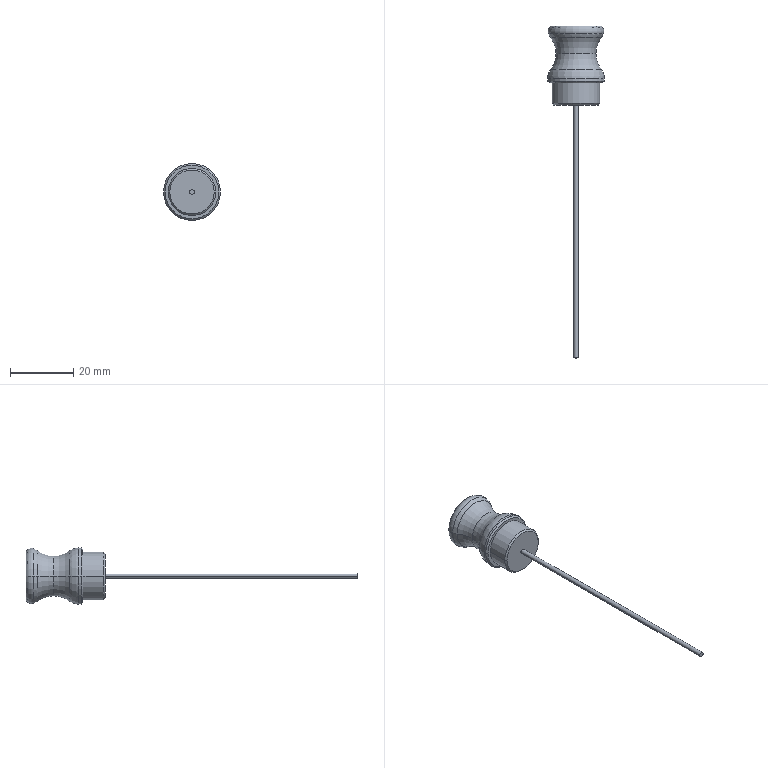Part | SolidWorks | features Chamfer 2, Fillet 1, Revolution 1 | 1 solid | 26 faces | box 18 x 105 x 18 mm | volume 4726 mm3 | torus 10 | cone 6 | cylinder 6 | plane 4 | commonest cylinder face diameters 1.5 x2 15 x2 18 x2
STEP:
#1=CARTESIAN_POINT('',(7.995,11.261,0.));
#2=VERTEX_POINT('',#1);
#3=CARTESIAN_POINT('',(6.308,16.305,0.));
#4=VERTEX_POINT('',#3);
#5=CARTESIAN_POINT('',(14.695,16.305,0.));
#6=DIRECTION('',(0.,0.,-1.));
#7=DIRECTION('',(-1.,0.,0.));
#8=AXIS2_PLACEMENT_3D('',#5,#6,#7);
#9=CIRCLE('',#8,8.387);
#10=EDGE_CURVE('',#2,#4,#9,.T.);
#11=ORIENTED_EDGE('',*,*,#10,.T.);
#12=CARTESIAN_POINT('',(-6.308,16.305,0.));
#13=VERTEX_POINT('',#12);
#14=CARTESIAN_POINT('',(0.,16.305,0.));
#15=DIRECTION('',(0.,-1.,0.));
#16=DIRECTION('',(1.,0.,0.));
#17=AXIS2_PLACEMENT_3D('',#14,#15,#16);
#18=CIRCLE('',#17,6.308);
#19=EDGE_CURVE('',#4,#13,#18,.T.);
#20=ORIENTED_EDGE('',*,*,#19,.T.);
#21=CARTESIAN_POINT('',(-7.995,11.261,0.));
#22=VERTEX_POINT('',#21);
#23=CARTESIAN_POINT('',(-14.695,16.305,0.));
#24=DIRECTION('',(0.,0.,1.));
#25=DIRECTION('',(1.,0.,0.));
#26=AXIS2_PLACEMENT_3D('',#23,#24,#25);
#27=CIRCLE('',#26,8.387);
#28=EDGE_CURVE('',#22,#13,#27,.T.);
#29=ORIENTED_EDGE('',*,*,#28,.F.);
#30=CARTESIAN_POINT('',(0.,11.261,0.));
#31=DIRECTION('',(0.,-1.,0.));
#32=DIRECTION('',(1.,0.,0.));
#33=AXIS2_PLACEMENT_3D('',#30,#31,#32);
#34=CIRCLE('',#33,7.995);
#35=EDGE_CURVE('',#2,#22,#34,.T.);
#36=ORIENTED_EDGE('',*,*,#35,.F.);
#37=EDGE_LOOP('',(#11,#20,#29,#36));
#38=FACE_OUTER_BOUND('',#37,.T.);
#39=CARTESIAN_POINT('',(0.,16.305,0.));
#40=DIRECTION('',(0.,-1.,0.));
#41=DIRECTION('',(1.,0.,0.));
#42=AXIS2_PLACEMENT_3D('',#39,#40,#41);
#43=TOROIDAL_SURFACE('',#42,14.695,8.387);
#44=ADVANCED_FACE('',(#38),#43,.F.);
#45=ORIENTED_EDGE('',*,*,#28,.T.);
#46=CARTESIAN_POINT('',(0.,16.305,0.));
#47=DIRECTION('',(0.,-1.,0.));
#48=DIRECTION('',(1.,0.,0.));
#49=AXIS2_PLACEMENT_3D('',#46,#47,#48);
#50=CIRCLE('',#49,6.308);
#51=EDGE_CURVE('',#13,#4,#50,.T.);
#52=ORIENTED_EDGE('',*,*,#51,.T.);
#53=ORIENTED_EDGE('',*,*,#10,.F.);
#54=CARTESIAN_POINT('',(0.,11.261,0.));
#55=DIRECTION('',(0.,-1.,0.));
#56=DIRECTION('',(1.,0.,0.));
#57=AXIS2_PLACEMENT_3D('',#54,#55,#56);
#58=CIRCLE('',#57,7.995);
#59=EDGE_CURVE('',#22,#2,#58,.T.);
#60=ORIENTED_EDGE('',*,*,#59,.F.);
#61=EDGE_LOOP('',(#45,#52,#53,#60));
#62=FACE_OUTER_BOUND('',#61,.T.);
#63=CARTESIAN_POINT('',(0.,16.305,0.));
#64=DIRECTION('',(0.,-1.,0.));
#65=DIRECTION('',(1.,0.,0.));
#66=AXIS2_PLACEMENT_3D('',#63,#64,#65);
#67=TOROIDAL_SURFACE('',#66,14.695,8.387);
#68=ADVANCED_FACE('',(#62),#67,.F.);
#69=CARTESIAN_POINT('',(8.69,22.623,0.));
#70=VERTEX_POINT('',#69);
#71=CARTESIAN_POINT('',(-8.69,22.623,0.));
#72=VERTEX_POINT('',#71);
#73=CARTESIAN_POINT('',(0.,22.623,0.));
#74=DIRECTION('',(0.,-1.,0.));
#75=DIRECTION('',(-1.,0.,0.));
#76=AXIS2_PLACEMENT_3D('',#73,#74,#75);
#77=CIRCLE('',#76,8.69);
#78=EDGE_CURVE('',#70,#72,#77,.T.);
#79=ORIENTED_EDGE('',*,*,#78,.F.);
#80=CARTESIAN_POINT('',(8.29,24.666,0.));
#81=VERTEX_POINT('',#80);
#82=CARTESIAN_POINT('',(6.814,23.316,0.));
#83=DIRECTION('',(0.,0.,1.));
#84=DIRECTION('',(1.,0.,0.));
#85=AXIS2_PLACEMENT_3D('',#82,#83,#84);
#86=CIRCLE('',#85,2.);
#87=EDGE_CURVE('',#70,#81,#86,.T.);
#88=ORIENTED_EDGE('',*,*,#87,.T.);
#89=CARTESIAN_POINT('',(-8.29,24.666,0.));
#90=VERTEX_POINT('',#89);
#91=CARTESIAN_POINT('',(0.,24.666,0.));
#92=DIRECTION('',(0.,1.,0.));
#93=DIRECTION('',(-1.,0.,0.));
#94=AXIS2_PLACEMENT_3D('',#91,#92,#93);
#95=CIRCLE('',#94,8.29);
#96=EDGE_CURVE('',#90,#81,#95,.T.);
#97=ORIENTED_EDGE('',*,*,#96,.F.);
#98=CARTESIAN_POINT('',(-6.814,23.316,0.));
#99=DIRECTION('',(0.,0.,-1.));
#100=DIRECTION('',(-1.,0.,0.));
#101=AXIS2_PLACEMENT_3D('',#98,#99,#100);
#102=CIRCLE('',#101,2.);
#103=EDGE_CURVE('',#72,#90,#102,.T.);
#104=ORIENTED_EDGE('',*,*,#103,.F.);
#105=EDGE_LOOP('',(#79,#88,#97,#104));
#106=FACE_OUTER_BOUND('',#105,.T.);
#107=CARTESIAN_POINT('',(0.,23.316,0.));
#108=DIRECTION('',(0.,1.,0.));
#109=DIRECTION('',(-1.,0.,0.));
#110=AXIS2_PLACEMENT_3D('',#107,#108,#109);
#111=TOROIDAL_SURFACE('',#110,6.814,2.);
#112=ADVANCED_FACE('',(#106),#111,.T.);
#113=CARTESIAN_POINT('',(7.,0.,0.));
#114=VERTEX_POINT('',#113);
#115=CARTESIAN_POINT('',(-7.,0.,0.));
#116=VERTEX_POINT('',#115);
#117=CARTESIAN_POINT('',(0.,0.,0.));
#118=DIRECTION('',(0.,-1.,0.));
#119=DIRECTION('',(1.,0.,0.));
#120=AXIS2_PLACEMENT_3D('',#117,#118,#119);
#121=CIRCLE('',#120,7.);
#122=EDGE_CURVE('',#114,#116,#121,.T.);
#123=ORIENTED_EDGE('',*,*,#122,.F.);
#124=CARTESIAN_POINT('',(7.5,0.5,0.));
#125=VERTEX_POINT('',#124);
#126=CARTESIAN_POINT('',(7.,0.,0.));
#127=DIRECTION('',(0.7071,0.7071,0.));
#128=VECTOR('',#127,1000.);
#129=LINE('',#126,#128);
#130=EDGE_CURVE('',#114,#125,#129,.T.);
#131=ORIENTED_EDGE('',*,*,#130,.T.);
#132=CARTESIAN_POINT('',(-7.5,0.5,0.));
#133=VERTEX_POINT('',#132);
#134=CARTESIAN_POINT('',(0.,0.5,0.));
#135=DIRECTION('',(0.,1.,0.));
#136=DIRECTION('',(1.,0.,0.));
#137=AXIS2_PLACEMENT_3D('',#134,#135,#136);
#138=CIRCLE('',#137,7.5);
#139=EDGE_CURVE('',#133,#125,#138,.T.);
#140=ORIENTED_EDGE('',*,*,#139,.F.);
#141=CARTESIAN_POINT('',(-7.,0.,0.));
#142=DIRECTION('',(-0.7071,0.7071,0.));
#143=VECTOR('',#142,1000.);
#144=LINE('',#141,#143);
#145=EDGE_CURVE('',#116,#133,#144,.T.);
#146=ORIENTED_EDGE('',*,*,#145,.F.);
#147=EDGE_LOOP('',(#123,#131,#140,#146));
#148=FACE_OUTER_BOUND('',#147,.T.);
#149=CARTESIAN_POINT('',(0.,0.,0.));
#150=DIRECTION('',(0.,1.,0.));
#151=DIRECTION('',(-1.,0.,0.));
#152=AXIS2_PLACEMENT_3D('',#149,#150,#151);
#153=CONICAL_SURFACE('',#152,7.,0.7854);
#154=ADVANCED_FACE('',(#148),#153,.T.);
#155=CARTESIAN_POINT('',(8.5,7.,0.));
#156=VERTEX_POINT('',#155);
#157=CARTESIAN_POINT('',(-8.5,7.,0.));
#158=VERTEX_POINT('',#157);
#159=CARTESIAN_POINT('',(0.,7.,0.));
#160=DIRECTION('',(0.,-1.,0.));
#161=DIRECTION('',(1.,0.,0.));
#162=AXIS2_PLACEMENT_3D('',#159,#160,#161);
#163=CIRCLE('',#162,8.5);
#164=EDGE_CURVE('',#156,#158,#163,.T.);
#165=ORIENTED_EDGE('',*,*,#164,.F.);
#166=CARTESIAN_POINT('',(9.,7.5,0.));
#167=VERTEX_POINT('',#166);
#168=CARTESIAN_POINT('',(8.5,7.,0.));
#169=DIRECTION('',(0.7071,0.7071,0.));
#170=VECTOR('',#169,1000.);
#171=LINE('',#168,#170);
#172=EDGE_CURVE('',#156,#167,#171,.T.);
#173=ORIENTED_EDGE('',*,*,#172,.T.);
#174=CARTESIAN_POINT('',(-9.,7.5,0.));
#175=VERTEX_POINT('',#174);
#176=CARTESIAN_POINT('',(0.,7.5,0.));
#177=DIRECTION('',(0.,1.,0.));
#178=DIRECTION('',(1.,0.,0.));
#179=AXIS2_PLACEMENT_3D('',#176,#177,#178);
#180=CIRCLE('',#179,9.);
#181=EDGE_CURVE('',#175,#167,#180,.T.);
#182=ORIENTED_EDGE('',*,*,#181,.F.);
#183=CARTESIAN_POINT('',(-8.5,7.,0.));
#184=DIRECTION('',(-0.7071,0.7071,0.));
#185=VECTOR('',#184,1000.);
#186=LINE('',#183,#185);
#187=EDGE_CURVE('',#158,#175,#186,.T.);
#188=ORIENTED_EDGE('',*,*,#187,.F.);
#189=EDGE_LOOP('',(#165,#173,#182,#188));
#190=FACE_OUTER_BOUND('',#189,.T.);
#191=CARTESIAN_POINT('',(0.,7.,0.));
#192=DIRECTION('',(0.,1.,0.));
#193=DIRECTION('',(-1.,0.,0.));
#194=AXIS2_PLACEMENT_3D('',#191,#192,#193);
#195=CONICAL_SURFACE('',#194,8.5,0.7854);
#196=ADVANCED_FACE('',(#190),#195,.T.);
#197=CARTESIAN_POINT('',(-7.984,25.,0.));
#198=VERTEX_POINT('',#197);
#199=CARTESIAN_POINT('',(7.984,25.,0.));
#200=VERTEX_POINT('',#199);
#201=CARTESIAN_POINT('',(0.,25.,0.));
#202=DIRECTION('',(0.,1.,0.));
#203=DIRECTION('',(-1.,0.,0.));
#204=AXIS2_PLACEMENT_3D('',#201,#202,#203);
#205=CIRCLE('',#204,7.984);
#206=EDGE_CURVE('',#198,#200,#205,.T.);
#207=ORIENTED_EDGE('',*,*,#206,.F.);
#208=CARTESIAN_POINT('',(-8.98,23.911,0.));
#209=DIRECTION('',(-0.675,-0.7379,0.));
#210=VECTOR('',#209,1000.);
#211=LINE('',#208,#210);
#212=EDGE_CURVE('',#198,#90,#211,.T.);
#213=ORIENTED_EDGE('',*,*,#212,.T.);
#214=ORIENTED_EDGE('',*,*,#96,.T.);
#215=CARTESIAN_POINT('',(8.98,23.911,0.));
#216=DIRECTION('',(0.675,-0.7379,0.));
#217=VECTOR('',#216,1000.);
#218=LINE('',#215,#217);
#219=EDGE_CURVE('',#200,#81,#218,.T.);
#220=ORIENTED_EDGE('',*,*,#219,.F.);
#221=EDGE_LOOP('',(#207,#213,#214,#220));
#222=FACE_OUTER_BOUND('',#221,.T.);
#223=CARTESIAN_POINT('',(0.,23.911,0.));
#224=DIRECTION('',(0.,-1.,0.));
#225=DIRECTION('',(1.,0.,0.));
#226=AXIS2_PLACEMENT_3D('',#223,#224,#225);
#227=CONICAL_SURFACE('',#226,8.98,0.7409);
#228=ADVANCED_FACE('',(#222),#227,.T.);
#229=CARTESIAN_POINT('',(0.75,0.,0.));
#230=VERTEX_POINT('',#229);
#231=CARTESIAN_POINT('',(-0.75,0.,0.));
#232=VERTEX_POINT('',#231);
#233=CARTESIAN_POINT('',(0.,0.,0.));
#234=DIRECTION('',(0.,-1.,0.));
#235=DIRECTION('',(1.,0.,0.));
#236=AXIS2_PLACEMENT_3D('',#233,#234,#235);
#237=CIRCLE('',#236,0.75);
#238=EDGE_CURVE('',#230,#232,#237,.T.);
#239=ORIENTED_EDGE('',*,*,#238,.T.);
#240=CARTESIAN_POINT('',(-0.75,-80.,0.));
#241=VERTEX_POINT('',#240);
#242=CARTESIAN_POINT('',(-0.75,-80.,0.));
#243=DIRECTION('',(0.,-1.,0.));
#244=VECTOR('',#243,1000.);
#245=LINE('',#242,#244);
#246=EDGE_CURVE('',#232,#241,#245,.T.);
#247=ORIENTED_EDGE('',*,*,#246,.T.);
#248=CARTESIAN_POINT('',(0.75,-80.,0.));
#249=VERTEX_POINT('',#248);
#250=CARTESIAN_POINT('',(0.,-80.,0.));
#251=DIRECTION('',(0.,-1.,0.));
#252=DIRECTION('',(1.,0.,0.));
#253=AXIS2_PLACEMENT_3D('',#250,#251,#252);
#254=CIRCLE('',#253,0.75);
#255=EDGE_CURVE('',#249,#241,#254,.T.);
#256=ORIENTED_EDGE('',*,*,#255,.F.);
#257=CARTESIAN_POINT('',(0.75,-80.,0.));
#258=DIRECTION('',(0.,-1.,0.));
#259=VECTOR('',#258,1000.);
#260=LINE('',#257,#259);
#261=EDGE_CURVE('',#230,#249,#260,.T.);
#262=ORIENTED_EDGE('',*,*,#261,.F.);
#263=EDGE_LOOP('',(#239,#247,#256,#262));
#264=FACE_OUTER_BOUND('',#263,.T.);
#265=CARTESIAN_POINT('',(0.,-80.,0.));
#266=DIRECTION('',(0.,-1.,0.));
#267=DIRECTION('',(1.,0.,0.));
#268=AXIS2_PLACEMENT_3D('',#265,#266,#267);
#269=CYLINDRICAL_SURFACE('',#268,0.75);
#270=ADVANCED_FACE('',(#264),#269,.T.);
#271=ORIENTED_EDGE('',*,*,#78,.T.);
#272=CARTESIAN_POINT('',(-7.995,21.348,0.));
#273=VERTEX_POINT('',#272);
#274=CARTESIAN_POINT('',(-4.,24.355,0.));
#275=DIRECTION('',(0.,0.,1.));
#276=DIRECTION('',(1.,0.,0.));
#277=AXIS2_PLACEMENT_3D('',#274,#275,#276);
#278=CIRCLE('',#277,5.);
#279=EDGE_CURVE('',#72,#273,#278,.T.);
#280=ORIENTED_EDGE('',*,*,#279,.T.);
#281=CARTESIAN_POINT('',(7.995,21.348,0.));
#282=VERTEX_POINT('',#281);
#283=CARTESIAN_POINT('',(0.,21.348,0.));
#284=DIRECTION('',(0.,-1.,0.));
#285=DIRECTION('',(1.,0.,0.));
#286=AXIS2_PLACEMENT_3D('',#283,#284,#285);
#287=CIRCLE('',#286,7.995);
#288=EDGE_CURVE('',#282,#273,#287,.T.);
#289=ORIENTED_EDGE('',*,*,#288,.F.);
#290=CARTESIAN_POINT('',(4.,24.355,0.));
#291=DIRECTION('',(0.,0.,-1.));
#292=DIRECTION('',(-1.,0.,0.));
#293=AXIS2_PLACEMENT_3D('',#290,#291,#292);
#294=CIRCLE('',#293,5.);
#295=EDGE_CURVE('',#70,#282,#294,.T.);
#296=ORIENTED_EDGE('',*,*,#295,.F.);
#297=EDGE_LOOP('',(#271,#280,#289,#296));
#298=FACE_OUTER_BOUND('',#297,.T.);
#299=CARTESIAN_POINT('',(0.,24.355,0.));
#300=DIRECTION('',(0.,-1.,0.));
#301=DIRECTION('',(1.,0.,0.));
#302=AXIS2_PLACEMENT_3D('',#299,#300,#301);
#303=TOROIDAL_SURFACE('',#302,4.,5.);
#304=ADVANCED_FACE('',(#298),#303,.T.);
#305=ORIENTED_EDGE('',*,*,#51,.F.);
#306=CARTESIAN_POINT('',(-14.695,16.305,0.));
#307=DIRECTION('',(0.,0.,1.));
#308=DIRECTION('',(1.,0.,0.));
#309=AXIS2_PLACEMENT_3D('',#306,#307,#308);
#310=CIRCLE('',#309,8.387);
#311=EDGE_CURVE('',#13,#273,#310,.T.);
#312=ORIENTED_EDGE('',*,*,#311,.T.);
#313=CARTESIAN_POINT('',(0.,21.348,0.));
#314=DIRECTION('',(0.,-1.,0.));
#315=DIRECTION('',(1.,0.,0.));
#316=AXIS2_PLACEMENT_3D('',#313,#314,#315);
#317=CIRCLE('',#316,7.995);
#318=EDGE_CURVE('',#273,#282,#317,.T.);
#319=ORIENTED_EDGE('',*,*,#318,.T.);
#320=CARTESIAN_POINT('',(14.695,16.305,0.));
#321=DIRECTION('',(0.,0.,-1.));
#322=DIRECTION('',(-1.,0.,0.));
#323=AXIS2_PLACEMENT_3D('',#320,#321,#322);
#324=CIRCLE('',#323,8.387);
#325=EDGE_CURVE('',#4,#282,#324,.T.);
#326=ORIENTED_EDGE('',*,*,#325,.F.);
#327=EDGE_LOOP('',(#305,#312,#319,#326));
#328=FACE_OUTER_BOUND('',#327,.T.);
#329=CARTESIAN_POINT('',(0.,16.305,0.));
#330=DIRECTION('',(0.,-1.,0.));
#331=DIRECTION('',(1.,0.,0.));
#332=AXIS2_PLACEMENT_3D('',#329,#330,#331);
#333=TOROIDAL_SURFACE('',#332,14.695,8.387);
#334=ADVANCED_FACE('',(#328),#333,.F.);
#335=ORIENTED_EDGE('',*,*,#35,.T.);
#336=CARTESIAN_POINT('',(-9.,8.254,0.));
#337=VERTEX_POINT('',#336);
#338=CARTESIAN_POINT('',(-4.,8.254,0.));
#339=DIRECTION('',(0.,0.,1.));
#340=DIRECTION('',(1.,0.,0.));
#341=AXIS2_PLACEMENT_3D('',#338,#339,#340);
#342=CIRCLE('',#341,5.);
#343=EDGE_CURVE('',#22,#337,#342,.T.);
#344=ORIENTED_EDGE('',*,*,#343,.T.);
#345=CARTESIAN_POINT('',(9.,8.254,0.));
#346=VERTEX_POINT('',#345);
#347=CARTESIAN_POINT('',(0.,8.254,0.));
#348=DIRECTION('',(0.,-1.,0.));
#349=DIRECTION('',(1.,0.,0.));
#350=AXIS2_PLACEMENT_3D('',#347,#348,#349);
#351=CIRCLE('',#350,9.);
#352=EDGE_CURVE('',#346,#337,#351,.T.);
#353=ORIENTED_EDGE('',*,*,#352,.F.);
#354=CARTESIAN_POINT('',(4.,8.254,0.));
#355=DIRECTION('',(0.,0.,-1.));
#356=DIRECTION('',(-1.,0.,0.));
#357=AXIS2_PLACEMENT_3D('',#354,#355,#356);
#358=CIRCLE('',#357,5.);
#359=EDGE_CURVE('',#2,#346,#358,.T.);
#360=ORIENTED_EDGE('',*,*,#359,.F.);
#361=EDGE_LOOP('',(#335,#344,#353,#360));
#362=FACE_OUTER_BOUND('',#361,.T.);
#363=CARTESIAN_POINT('',(0.,8.254,0.));
#364=DIRECTION('',(0.,-1.,0.));
#365=DIRECTION('',(1.,0.,0.));
#366=AXIS2_PLACEMENT_3D('',#363,#364,#365);
#367=TOROIDAL_SURFACE('',#366,4.,5.);
#368=ADVANCED_FACE('',(#362),#367,.T.);
#369=ORIENTED_EDGE('',*,*,#352,.T.);
#370=CARTESIAN_POINT('',(-9.,-80.,0.));
#371=DIRECTION('',(0.,-1.,0.));
#372=VECTOR('',#371,1000.);
#373=LINE('',#370,#372);
#374=EDGE_CURVE('',#337,#175,#373,.T.);
#375=ORIENTED_EDGE('',*,*,#374,.T.);
#376=ORIENTED_EDGE('',*,*,#181,.T.);
#377=CARTESIAN_POINT('',(9.,-80.,0.));
#378=DIRECTION('',(0.,-1.,0.));
#379=VECTOR('',#378,1000.);
#380=LINE('',#377,#379);
#381=EDGE_CURVE('',#346,#167,#380,.T.);
#382=ORIENTED_EDGE('',*,*,#381,.F.);
#383=EDGE_LOOP('',(#369,#375,#376,#382));
#384=FACE_OUTER_BOUND('',#383,.T.);
#385=CARTESIAN_POINT('',(0.,-80.,0.));
#386=DIRECTION('',(0.,-1.,0.));
#387=DIRECTION('',(1.,0.,0.));
#388=AXIS2_PLACEMENT_3D('',#385,#386,#387);
#389=CYLINDRICAL_SURFACE('',#388,9.);
#390=ADVANCED_FACE('',(#384),#389,.T.);
#391=CARTESIAN_POINT('',(7.5,7.,0.));
#392=VERTEX_POINT('',#391);
#393=CARTESIAN_POINT('',(-7.5,7.,0.));
#394=VERTEX_POINT('',#393);
#395=CARTESIAN_POINT('',(0.,7.,0.));
#396=DIRECTION('',(0.,-1.,0.));
#397=DIRECTION('',(1.,0.,0.));
#398=AXIS2_PLACEMENT_3D('',#395,#396,#397);
#399=CIRCLE('',#398,7.5);
#400=EDGE_CURVE('',#392,#394,#399,.T.);
#401=ORIENTED_EDGE('',*,*,#400,.T.);
#402=CARTESIAN_POINT('',(-7.5,-80.,0.));
#403=DIRECTION('',(0.,-1.,0.));
#404=VECTOR('',#403,1000.);
#405=LINE('',#402,#404);
#406=EDGE_CURVE('',#394,#133,#405,.T.);
#407=ORIENTED_EDGE('',*,*,#406,.T.);
#408=ORIENTED_EDGE('',*,*,#139,.T.);
#409=CARTESIAN_POINT('',(7.5,-80.,0.));
#410=DIRECTION('',(0.,-1.,0.));
#411=VECTOR('',#410,1000.);
#412=LINE('',#409,#411);
#413=EDGE_CURVE('',#392,#125,#412,.T.);
#414=ORIENTED_EDGE('',*,*,#413,.F.);
#415=EDGE_LOOP('',(#401,#407,#408,#414));
#416=FACE_OUTER_BOUND('',#415,.T.);
#417=CARTESIAN_POINT('',(0.,-80.,0.));
#418=DIRECTION('',(0.,-1.,0.));
#419=DIRECTION('',(1.,0.,0.));
#420=AXIS2_PLACEMENT_3D('',#417,#418,#419);
#421=CYLINDRICAL_SURFACE('',#420,7.5);
#422=ADVANCED_FACE('',(#416),#421,.T.);
#423=ORIENTED_EDGE('',*,*,#406,.F.);
#424=CARTESIAN_POINT('',(0.,7.,0.));
#425=DIRECTION('',(0.,-1.,0.));
#426=DIRECTION('',(1.,0.,0.));
#427=AXIS2_PLACEMENT_3D('',#424,#425,#426);
#428=CIRCLE('',#427,7.5);
#429=EDGE_CURVE('',#394,#392,#428,.T.);
#430=ORIENTED_EDGE('',*,*,#429,.T.);
#431=ORIENTED_EDGE('',*,*,#413,.T.);
#432=CARTESIAN_POINT('',(0.,0.5,0.));
#433=DIRECTION('',(0.,1.,0.));
#434=DIRECTION('',(1.,0.,0.));
#435=AXIS2_PLACEMENT_3D('',#432,#433,#434);
#436=CIRCLE('',#435,7.5);
#437=EDGE_CURVE('',#125,#133,#436,.T.);
#438=ORIENTED_EDGE('',*,*,#437,.T.);
#439=EDGE_LOOP('',(#423,#430,#431,#438));
#440=FACE_OUTER_BOUND('',#439,.T.);
#441=CARTESIAN_POINT('',(0.,-80.,0.));
#442=DIRECTION('',(0.,-1.,0.));
#443=DIRECTION('',(1.,0.,0.));
#444=AXIS2_PLACEMENT_3D('',#441,#442,#443);
#445=CYLINDRICAL_SURFACE('',#444,7.5);
#446=ADVANCED_FACE('',(#440),#445,.T.);
#447=CARTESIAN_POINT('',(0.,7.,0.));
#448=DIRECTION('',(0.,-1.,0.));
#449=DIRECTION('',(1.,0.,0.));
#450=AXIS2_PLACEMENT_3D('',#447,#448,#449);
#451=CIRCLE('',#450,8.5);
#452=EDGE_CURVE('',#158,#156,#451,.T.);
#453=ORIENTED_EDGE('',*,*,#452,.T.);
#454=ORIENTED_EDGE('',*,*,#164,.T.);
#455=EDGE_LOOP('',(#453,#454));
#456=FACE_OUTER_BOUND('',#455,.T.);
#457=ORIENTED_EDGE('',*,*,#400,.F.);
#458=ORIENTED_EDGE('',*,*,#429,.F.);
#459=EDGE_LOOP('',(#457,#458));
#460=FACE_BOUND('',#459,.T.);
#461=CARTESIAN_POINT('',(7.5,7.,0.));
#462=DIRECTION('',(0.,-1.,0.));
#463=DIRECTION('',(1.,0.,0.));
#464=AXIS2_PLACEMENT_3D('',#461,#462,#463);
#465=PLANE('',#464);
#466=ADVANCED_FACE('',(#456,#460),#465,.T.);
#467=ORIENTED_EDGE('',*,*,#374,.F.);
#468=CARTESIAN_POINT('',(0.,8.254,0.));
#469=DIRECTION('',(0.,-1.,0.));
#470=DIRECTION('',(1.,0.,0.));
#471=AXIS2_PLACEMENT_3D('',#468,#469,#470);
#472=CIRCLE('',#471,9.);
#473=EDGE_CURVE('',#337,#346,#472,.T.);
#474=ORIENTED_EDGE('',*,*,#473,.T.);
#475=ORIENTED_EDGE('',*,*,#381,.T.);
#476=CARTESIAN_POINT('',(0.,7.5,0.));
#477=DIRECTION('',(0.,1.,0.));
#478=DIRECTION('',(1.,0.,0.));
#479=AXIS2_PLACEMENT_3D('',#476,#477,#478);
#480=CIRCLE('',#479,9.);
#481=EDGE_CURVE('',#167,#175,#480,.T.);
#482=ORIENTED_EDGE('',*,*,#481,.T.);
#483=EDGE_LOOP('',(#467,#474,#475,#482));
#484=FACE_OUTER_BOUND('',#483,.T.);
#485=CARTESIAN_POINT('',(0.,-80.,0.));
#486=DIRECTION('',(0.,-1.,0.));
#487=DIRECTION('',(1.,0.,0.));
#488=AXIS2_PLACEMENT_3D('',#485,#486,#487);
#489=CYLINDRICAL_SURFACE('',#488,9.);
#490=ADVANCED_FACE('',(#484),#489,.T.);
#491=ORIENTED_EDGE('',*,*,#343,.F.);
#492=ORIENTED_EDGE('',*,*,#59,.T.);
#493=ORIENTED_EDGE('',*,*,#359,.T.);
#494=ORIENTED_EDGE('',*,*,#473,.F.);
#495=EDGE_LOOP('',(#491,#492,#493,#494));
#496=FACE_OUTER_BOUND('',#495,.T.);
#497=CARTESIAN_POINT('',(0.,8.254,0.));
#498=DIRECTION('',(0.,-1.,0.));
#499=DIRECTION('',(1.,0.,0.));
#500=AXIS2_PLACEMENT_3D('',#497,#498,#499);
#501=TOROIDAL_SURFACE('',#500,4.,5.);
#502=ADVANCED_FACE('',(#496),#501,.T.);
#503=ORIENTED_EDGE('',*,*,#19,.F.);
#504=ORIENTED_EDGE('',*,*,#325,.T.);
#505=ORIENTED_EDGE('',*,*,#288,.T.);
#506=ORIENTED_EDGE('',*,*,#311,.F.);
#507=EDGE_LOOP('',(#503,#504,#505,#506));
#508=FACE_OUTER_BOUND('',#507,.T.);
#509=CARTESIAN_POINT('',(0.,16.305,0.));
#510=DIRECTION('',(0.,-1.,0.));
#511=DIRECTION('',(1.,0.,0.));
#512=AXIS2_PLACEMENT_3D('',#509,#510,#511);
#513=TOROIDAL_SURFACE('',#512,14.695,8.387);
#514=ADVANCED_FACE('',(#508),#513,.F.);
#515=ORIENTED_EDGE('',*,*,#279,.F.);
#516=CARTESIAN_POINT('',(0.,22.623,0.));
#517=DIRECTION('',(0.,-1.,0.));
#518=DIRECTION('',(-1.,0.,0.));
#519=AXIS2_PLACEMENT_3D('',#516,#517,#518);
#520=CIRCLE('',#519,8.69);
#521=EDGE_CURVE('',#72,#70,#520,.T.);
#522=ORIENTED_EDGE('',*,*,#521,.T.);
#523=ORIENTED_EDGE('',*,*,#295,.T.);
#524=ORIENTED_EDGE('',*,*,#318,.F.);
#525=EDGE_LOOP('',(#515,#522,#523,#524));
#526=FACE_OUTER_BOUND('',#525,.T.);
#527=CARTESIAN_POINT('',(0.,24.355,0.));
#528=DIRECTION('',(0.,-1.,0.));
#529=DIRECTION('',(1.,0.,0.));
#530=AXIS2_PLACEMENT_3D('',#527,#528,#529);
#531=TOROIDAL_SURFACE('',#530,4.,5.);
#532=ADVANCED_FACE('',(#526),#531,.T.);
#533=CARTESIAN_POINT('',(0.,25.,0.));
#534=DIRECTION('',(0.,1.,0.));
#535=DIRECTION('',(-1.,0.,0.));
#536=AXIS2_PLACEMENT_3D('',#533,#534,#535);
#537=CIRCLE('',#536,7.984);
#538=EDGE_CURVE('',#200,#198,#537,.T.);
#539=ORIENTED_EDGE('',*,*,#538,.T.);
#540=ORIENTED_EDGE('',*,*,#206,.T.);
#541=EDGE_LOOP('',(#539,#540));
#542=FACE_OUTER_BOUND('',#541,.T.);
#543=CARTESIAN_POINT('',(9.,25.,0.));
#544=DIRECTION('',(0.,1.,0.));
#545=DIRECTION('',(-1.,0.,0.));
#546=AXIS2_PLACEMENT_3D('',#543,#544,#545);
#547=PLANE('',#546);
#548=ADVANCED_FACE('',(#542),#547,.T.);
#549=ORIENTED_EDGE('',*,*,#255,.T.);
#550=CARTESIAN_POINT('',(0.,-80.,0.));
#551=DIRECTION('',(0.,-1.,0.));
#552=DIRECTION('',(1.,0.,0.));
#553=AXIS2_PLACEMENT_3D('',#550,#551,#552);
#554=CIRCLE('',#553,0.75);
#555=EDGE_CURVE('',#241,#249,#554,.T.);
#556=ORIENTED_EDGE('',*,*,#555,.T.);
#557=EDGE_LOOP('',(#549,#556));
#558=FACE_OUTER_BOUND('',#557,.T.);
#559=CARTESIAN_POINT('',(0.,-80.,0.));
#560=DIRECTION('',(0.,-1.,0.));
#561=DIRECTION('',(1.,0.,0.));
#562=AXIS2_PLACEMENT_3D('',#559,#560,#561);
#563=PLANE('',#562);
#564=ADVANCED_FACE('',(#558),#563,.T.);
#565=ORIENTED_EDGE('',*,*,#246,.F.);
#566=CARTESIAN_POINT('',(0.,0.,0.));
#567=DIRECTION('',(0.,-1.,0.));
#568=DIRECTION('',(1.,0.,0.));
#569=AXIS2_PLACEMENT_3D('',#566,#567,#568);
#570=CIRCLE('',#569,0.75);
#571=EDGE_CURVE('',#232,#230,#570,.T.);
#572=ORIENTED_EDGE('',*,*,#571,.T.);
#573=ORIENTED_EDGE('',*,*,#261,.T.);
#574=ORIENTED_EDGE('',*,*,#555,.F.);
#575=EDGE_LOOP('',(#565,#572,#573,#574));
#576=FACE_OUTER_BOUND('',#575,.T.);
#577=CARTESIAN_POINT('',(0.,-80.,0.));
#578=DIRECTION('',(0.,-1.,0.));
#579=DIRECTION('',(1.,0.,0.));
#580=AXIS2_PLACEMENT_3D('',#577,#578,#579);
#581=CYLINDRICAL_SURFACE('',#580,0.75);
#582=ADVANCED_FACE('',(#576),#581,.T.);
#583=CARTESIAN_POINT('',(0.,0.,0.));
#584=DIRECTION('',(0.,-1.,0.));
#585=DIRECTION('',(1.,0.,0.));
#586=AXIS2_PLACEMENT_3D('',#583,#584,#585);
#587=CIRCLE('',#586,7.);
#588=EDGE_CURVE('',#116,#114,#587,.T.);
#589=ORIENTED_EDGE('',*,*,#588,.T.);
#590=ORIENTED_EDGE('',*,*,#122,.T.);
#591=EDGE_LOOP('',(#589,#590));
#592=FACE_OUTER_BOUND('',#591,.T.);
#593=ORIENTED_EDGE('',*,*,#238,.F.);
#594=ORIENTED_EDGE('',*,*,#571,.F.);
#595=EDGE_LOOP('',(#593,#594));
#596=FACE_BOUND('',#595,.T.);
#597=CARTESIAN_POINT('',(0.75,0.,0.));
#598=DIRECTION('',(0.,-1.,0.));
#599=DIRECTION('',(1.,0.,0.));
#600=AXIS2_PLACEMENT_3D('',#597,#598,#599);
#601=PLANE('',#600);
#602=ADVANCED_FACE('',(#592,#596),#601,.T.);
#603=ORIENTED_EDGE('',*,*,#212,.F.);
#604=ORIENTED_EDGE('',*,*,#538,.F.);
#605=ORIENTED_EDGE('',*,*,#219,.T.);
#606=CARTESIAN_POINT('',(0.,24.666,0.));
#607=DIRECTION('',(0.,1.,0.));
#608=DIRECTION('',(-1.,0.,0.));
#609=AXIS2_PLACEMENT_3D('',#606,#607,#608);
#610=CIRCLE('',#609,8.29);
#611=EDGE_CURVE('',#81,#90,#610,.T.);
#612=ORIENTED_EDGE('',*,*,#611,.T.);
#613=EDGE_LOOP('',(#603,#604,#605,#612));
#614=FACE_OUTER_BOUND('',#613,.T.);
#615=CARTESIAN_POINT('',(0.,23.911,0.));
#616=DIRECTION('',(0.,-1.,0.));
#617=DIRECTION('',(1.,0.,0.));
#618=AXIS2_PLACEMENT_3D('',#615,#616,#617);
#619=CONICAL_SURFACE('',#618,8.98,0.7409);
#620=ADVANCED_FACE('',(#614),#619,.T.);
#621=ORIENTED_EDGE('',*,*,#172,.F.);
#622=ORIENTED_EDGE('',*,*,#452,.F.);
#623=ORIENTED_EDGE('',*,*,#187,.T.);
#624=ORIENTED_EDGE('',*,*,#481,.F.);
#625=EDGE_LOOP('',(#621,#622,#623,#624));
#626=FACE_OUTER_BOUND('',#625,.T.);
#627=CARTESIAN_POINT('',(0.,7.,0.));
#628=DIRECTION('',(0.,1.,0.));
#629=DIRECTION('',(-1.,0.,0.));
#630=AXIS2_PLACEMENT_3D('',#627,#628,#629);
#631=CONICAL_SURFACE('',#630,8.5,0.7854);
#632=ADVANCED_FACE('',(#626),#631,.T.);
#633=ORIENTED_EDGE('',*,*,#130,.F.);
#634=ORIENTED_EDGE('',*,*,#588,.F.);
#635=ORIENTED_EDGE('',*,*,#145,.T.);
#636=ORIENTED_EDGE('',*,*,#437,.F.);
#637=EDGE_LOOP('',(#633,#634,#635,#636));
#638=FACE_OUTER_BOUND('',#637,.T.);
#639=CARTESIAN_POINT('',(0.,0.,0.));
#640=DIRECTION('',(0.,1.,0.));
#641=DIRECTION('',(-1.,0.,0.));
#642=AXIS2_PLACEMENT_3D('',#639,#640,#641);
#643=CONICAL_SURFACE('',#642,7.,0.7854);
#644=ADVANCED_FACE('',(#638),#643,.T.);
#645=ORIENTED_EDGE('',*,*,#87,.F.);
#646=ORIENTED_EDGE('',*,*,#521,.F.);
#647=ORIENTED_EDGE('',*,*,#103,.T.);
#648=ORIENTED_EDGE('',*,*,#611,.F.);
#649=EDGE_LOOP('',(#645,#646,#647,#648));
#650=FACE_OUTER_BOUND('',#649,.T.);
#651=CARTESIAN_POINT('',(0.,23.316,0.));
#652=DIRECTION('',(0.,1.,0.));
#653=DIRECTION('',(-1.,0.,0.));
#654=AXIS2_PLACEMENT_3D('',#651,#652,#653);
#655=TOROIDAL_SURFACE('',#654,6.814,2.);
#656=ADVANCED_FACE('',(#650),#655,.T.);
#657=CLOSED_SHELL('',(#44,#68,#112,#154,#196,#228,#270,#304,#334,#368,#390,#422,#446,#466,#490,#502,#514,#532,#548,#564,#582,#602,#620,#632,#644,#656));
#658=MANIFOLD_SOLID_BREP('',#657);
#659=CARTESIAN_POINT('',(0.,0.,0.));
#660=DIRECTION('',(0.,0.,1.));
#661=DIRECTION('',(1.,0.,0.));
#662=AXIS2_PLACEMENT_3D('',#659,#660,#661);
#663=(LENGTH_UNIT()NAMED_UNIT(*)SI_UNIT(.MILLI.,.METRE.));
#664=UNCERTAINTY_MEASURE_WITH_UNIT(LENGTH_MEASURE(0.00001),#663,'','');
#665=(NAMED_UNIT(*)PLANE_ANGLE_UNIT()SI_UNIT($,.RADIAN.));
#666=(NAMED_UNIT(*)SI_UNIT($,.STERADIAN.)SOLID_ANGLE_UNIT());
#667=(GEOMETRIC_REPRESENTATION_CONTEXT(3)GLOBAL_UNCERTAINTY_ASSIGNED_CONTEXT((#664))GLOBAL_UNIT_ASSIGNED_CONTEXT((#663,#665,#666))REPRESENTATION_CONTEXT('',''));
#668=ADVANCED_BREP_SHAPE_REPRESENTATION('',(#658,#662),#667);